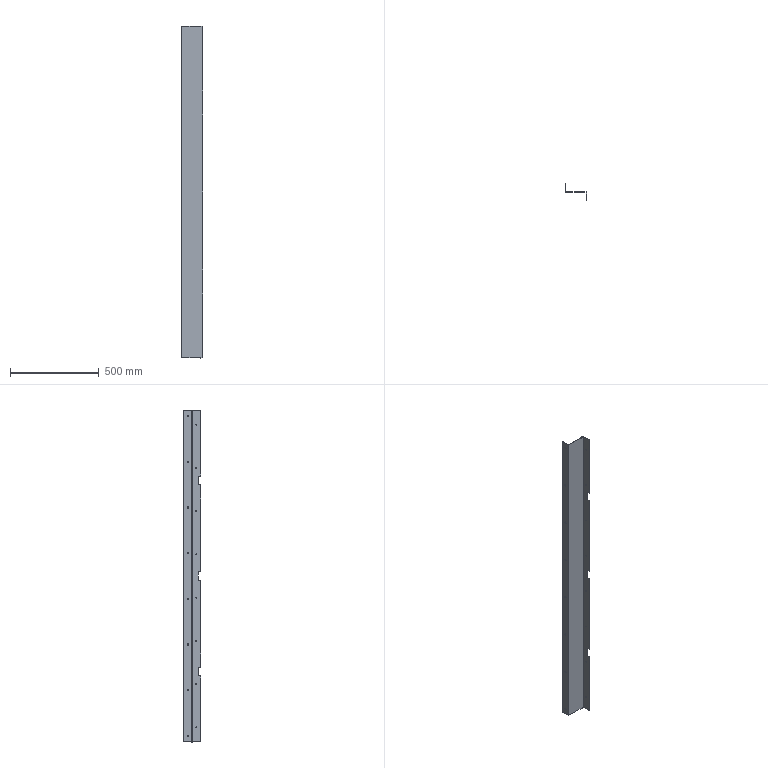Part | STEP file | SX-003-02 | 1 solid | 74 faces | box 120 x 98 x 1870 mm | volume 796406 mm3 | plane 38 | cylinder 36 | commonest cylinder face diameters 5.4 x16 8 x16 0.4 x2 4.4 x2